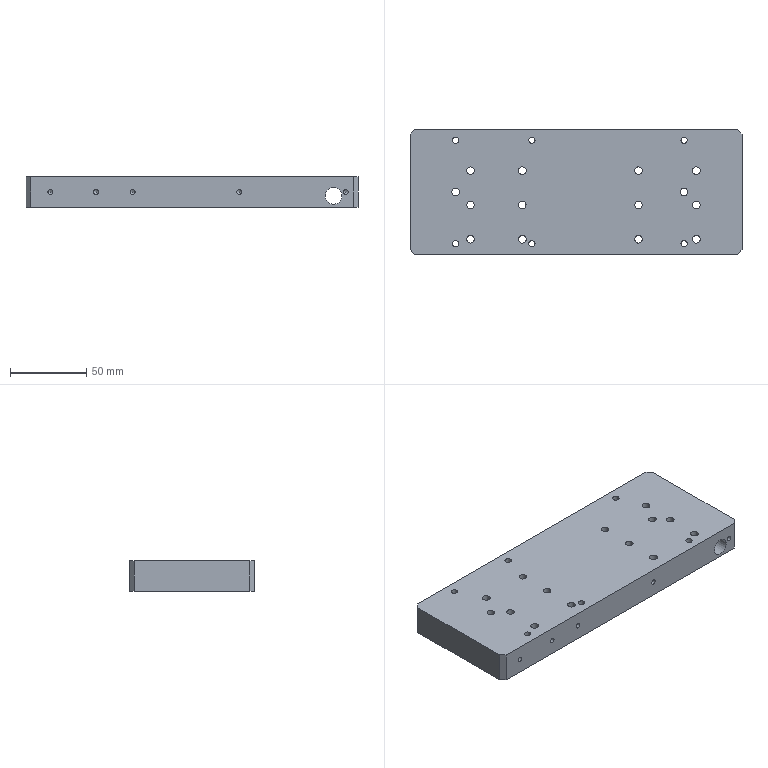Part | 1 solid | 49 faces | box 218 x 82 x 20 mm | volume 338244 mm3 | cylinder 30 | plane 10 | cone 9 | commonest cylinder face diameters 5.1 x8 4.2 x6 5 x6 3.3 x5 6.8 x4 11 x1
STEP:
#1=CARTESIAN_POINT('',(-109.,-38.,10.));
#2=VERTEX_POINT('',#1);
#3=CARTESIAN_POINT('',(-106.,-41.,10.));
#4=VERTEX_POINT('',#3);
#5=CARTESIAN_POINT('',(-106.,-41.,10.));
#6=DIRECTION('',(0.7071,-0.7071,0.));
#7=VECTOR('',#6,1000.);
#8=LINE('',#5,#7);
#9=EDGE_CURVE('',#2,#4,#8,.T.);
#10=ORIENTED_EDGE('',*,*,#9,.F.);
#11=CARTESIAN_POINT('',(-109.,-38.,-10.));
#12=VERTEX_POINT('',#11);
#13=CARTESIAN_POINT('',(-109.,-38.,10.));
#14=DIRECTION('',(0.,0.,1.));
#15=VECTOR('',#14,1000.);
#16=LINE('',#13,#15);
#17=EDGE_CURVE('',#12,#2,#16,.T.);
#18=ORIENTED_EDGE('',*,*,#17,.F.);
#19=CARTESIAN_POINT('',(-106.,-41.,-10.));
#20=VERTEX_POINT('',#19);
#21=CARTESIAN_POINT('',(-73.5,-73.5,-10.));
#22=DIRECTION('',(-0.7071,0.7071,0.));
#23=VECTOR('',#22,1000.);
#24=LINE('',#21,#23);
#25=EDGE_CURVE('',#20,#12,#24,.T.);
#26=ORIENTED_EDGE('',*,*,#25,.F.);
#27=CARTESIAN_POINT('',(-106.,-41.,-10.));
#28=DIRECTION('',(0.,0.,-1.));
#29=VECTOR('',#28,1000.);
#30=LINE('',#27,#29);
#31=EDGE_CURVE('',#4,#20,#30,.T.);
#32=ORIENTED_EDGE('',*,*,#31,.F.);
#33=EDGE_LOOP('',(#10,#18,#26,#32));
#34=FACE_BOUND('',#33,.T.);
#35=CARTESIAN_POINT('',(-106.,-41.,10.));
#36=DIRECTION('',(-0.7071,-0.7071,0.));
#37=DIRECTION('',(0.,0.,1.));
#38=AXIS2_PLACEMENT_3D('',#35,#36,#37);
#39=PLANE('',#38);
#40=ADVANCED_FACE('',(#34),#39,.T.);
#41=CARTESIAN_POINT('',(106.,-41.,10.));
#42=VERTEX_POINT('',#41);
#43=CARTESIAN_POINT('',(109.,-38.,10.));
#44=VERTEX_POINT('',#43);
#45=CARTESIAN_POINT('',(109.,-38.,10.));
#46=DIRECTION('',(0.7071,0.7071,0.));
#47=VECTOR('',#46,1000.);
#48=LINE('',#45,#47);
#49=EDGE_CURVE('',#42,#44,#48,.T.);
#50=ORIENTED_EDGE('',*,*,#49,.F.);
#51=CARTESIAN_POINT('',(106.,-41.,-10.));
#52=VERTEX_POINT('',#51);
#53=CARTESIAN_POINT('',(106.,-41.,10.));
#54=DIRECTION('',(0.,0.,1.));
#55=VECTOR('',#54,1000.);
#56=LINE('',#53,#55);
#57=EDGE_CURVE('',#52,#42,#56,.T.);
#58=ORIENTED_EDGE('',*,*,#57,.F.);
#59=CARTESIAN_POINT('',(109.,-38.,-10.));
#60=VERTEX_POINT('',#59);
#61=CARTESIAN_POINT('',(73.5,-73.5,-10.));
#62=DIRECTION('',(-0.7071,-0.7071,0.));
#63=VECTOR('',#62,1000.);
#64=LINE('',#61,#63);
#65=EDGE_CURVE('',#60,#52,#64,.T.);
#66=ORIENTED_EDGE('',*,*,#65,.F.);
#67=CARTESIAN_POINT('',(109.,-38.,10.));
#68=DIRECTION('',(0.,0.,-1.));
#69=VECTOR('',#68,1000.);
#70=LINE('',#67,#69);
#71=EDGE_CURVE('',#44,#60,#70,.T.);
#72=ORIENTED_EDGE('',*,*,#71,.F.);
#73=EDGE_LOOP('',(#50,#58,#66,#72));
#74=FACE_BOUND('',#73,.T.);
#75=CARTESIAN_POINT('',(109.,-38.,10.));
#76=DIRECTION('',(-0.7071,0.7071,0.));
#77=DIRECTION('',(0.,0.,-1.));
#78=AXIS2_PLACEMENT_3D('',#75,#76,#77);
#79=PLANE('',#78);
#80=ADVANCED_FACE('',(#74),#79,.F.);
#81=CARTESIAN_POINT('',(-106.,41.,10.));
#82=VERTEX_POINT('',#81);
#83=CARTESIAN_POINT('',(-109.,38.,10.));
#84=VERTEX_POINT('',#83);
#85=CARTESIAN_POINT('',(-109.,38.,10.));
#86=DIRECTION('',(-0.7071,-0.7071,0.));
#87=VECTOR('',#86,1000.);
#88=LINE('',#85,#87);
#89=EDGE_CURVE('',#82,#84,#88,.T.);
#90=ORIENTED_EDGE('',*,*,#89,.F.);
#91=CARTESIAN_POINT('',(-106.,41.,-10.));
#92=VERTEX_POINT('',#91);
#93=CARTESIAN_POINT('',(-106.,41.,10.));
#94=DIRECTION('',(0.,0.,1.));
#95=VECTOR('',#94,1000.);
#96=LINE('',#93,#95);
#97=EDGE_CURVE('',#92,#82,#96,.T.);
#98=ORIENTED_EDGE('',*,*,#97,.F.);
#99=CARTESIAN_POINT('',(-109.,38.,-10.));
#100=VERTEX_POINT('',#99);
#101=CARTESIAN_POINT('',(-73.5,73.5,-10.));
#102=DIRECTION('',(0.7071,0.7071,0.));
#103=VECTOR('',#102,1000.);
#104=LINE('',#101,#103);
#105=EDGE_CURVE('',#100,#92,#104,.T.);
#106=ORIENTED_EDGE('',*,*,#105,.F.);
#107=CARTESIAN_POINT('',(-109.,38.,10.));
#108=DIRECTION('',(0.,0.,-1.));
#109=VECTOR('',#108,1000.);
#110=LINE('',#107,#109);
#111=EDGE_CURVE('',#84,#100,#110,.T.);
#112=ORIENTED_EDGE('',*,*,#111,.F.);
#113=EDGE_LOOP('',(#90,#98,#106,#112));
#114=FACE_BOUND('',#113,.T.);
#115=CARTESIAN_POINT('',(-109.,38.,10.));
#116=DIRECTION('',(0.7071,-0.7071,0.));
#117=DIRECTION('',(0.,0.,-1.));
#118=AXIS2_PLACEMENT_3D('',#115,#116,#117);
#119=PLANE('',#118);
#120=ADVANCED_FACE('',(#114),#119,.F.);
#121=CARTESIAN_POINT('',(109.,38.,10.));
#122=VERTEX_POINT('',#121);
#123=CARTESIAN_POINT('',(106.,41.,10.));
#124=VERTEX_POINT('',#123);
#125=CARTESIAN_POINT('',(106.,41.,10.));
#126=DIRECTION('',(-0.7071,0.7071,0.));
#127=VECTOR('',#126,1000.);
#128=LINE('',#125,#127);
#129=EDGE_CURVE('',#122,#124,#128,.T.);
#130=ORIENTED_EDGE('',*,*,#129,.F.);
#131=CARTESIAN_POINT('',(109.,38.,-10.));
#132=VERTEX_POINT('',#131);
#133=CARTESIAN_POINT('',(109.,38.,10.));
#134=DIRECTION('',(0.,0.,1.));
#135=VECTOR('',#134,1000.);
#136=LINE('',#133,#135);
#137=EDGE_CURVE('',#132,#122,#136,.T.);
#138=ORIENTED_EDGE('',*,*,#137,.F.);
#139=CARTESIAN_POINT('',(106.,41.,-10.));
#140=VERTEX_POINT('',#139);
#141=CARTESIAN_POINT('',(73.5,73.5,-10.));
#142=DIRECTION('',(0.7071,-0.7071,0.));
#143=VECTOR('',#142,1000.);
#144=LINE('',#141,#143);
#145=EDGE_CURVE('',#140,#132,#144,.T.);
#146=ORIENTED_EDGE('',*,*,#145,.F.);
#147=CARTESIAN_POINT('',(106.,41.,-10.));
#148=DIRECTION('',(0.,0.,-1.));
#149=VECTOR('',#148,1000.);
#150=LINE('',#147,#149);
#151=EDGE_CURVE('',#124,#140,#150,.T.);
#152=ORIENTED_EDGE('',*,*,#151,.F.);
#153=EDGE_LOOP('',(#130,#138,#146,#152));
#154=FACE_BOUND('',#153,.T.);
#155=CARTESIAN_POINT('',(106.,41.,10.));
#156=DIRECTION('',(0.7071,0.7071,0.));
#157=DIRECTION('',(0.,0.,1.));
#158=AXIS2_PLACEMENT_3D('',#155,#156,#157);
#159=PLANE('',#158);
#160=ADVANCED_FACE('',(#154),#159,.T.);
#161=CARTESIAN_POINT('',(-109.,41.,-10.));
#162=DIRECTION('',(1.,0.,0.));
#163=VECTOR('',#162,1000.);
#164=LINE('',#161,#163);
#165=EDGE_CURVE('',#92,#140,#164,.T.);
#166=ORIENTED_EDGE('',*,*,#165,.T.);
#167=ORIENTED_EDGE('',*,*,#145,.T.);
#168=CARTESIAN_POINT('',(109.,-41.,-10.));
#169=DIRECTION('',(0.,1.,0.));
#170=VECTOR('',#169,1000.);
#171=LINE('',#168,#170);
#172=EDGE_CURVE('',#60,#132,#171,.T.);
#173=ORIENTED_EDGE('',*,*,#172,.F.);
#174=ORIENTED_EDGE('',*,*,#65,.T.);
#175=CARTESIAN_POINT('',(-109.,-41.,-10.));
#176=DIRECTION('',(1.,0.,0.));
#177=VECTOR('',#176,1000.);
#178=LINE('',#175,#177);
#179=EDGE_CURVE('',#20,#52,#178,.T.);
#180=ORIENTED_EDGE('',*,*,#179,.F.);
#181=ORIENTED_EDGE('',*,*,#25,.T.);
#182=CARTESIAN_POINT('',(-109.,-41.,-10.));
#183=DIRECTION('',(0.,1.,0.));
#184=VECTOR('',#183,1000.);
#185=LINE('',#182,#184);
#186=EDGE_CURVE('',#12,#100,#185,.T.);
#187=ORIENTED_EDGE('',*,*,#186,.T.);
#188=ORIENTED_EDGE('',*,*,#105,.T.);
#189=EDGE_LOOP('',(#166,#167,#173,#174,#180,#181,#187,#188));
#190=FACE_BOUND('',#189,.T.);
#191=CARTESIAN_POINT('',(38.45,14.,-10.));
#192=VERTEX_POINT('',#191);
#193=CARTESIAN_POINT('',(41.,14.,-10.));
#194=DIRECTION('',(0.,0.,-1.));
#195=DIRECTION('',(-1.,0.,0.));
#196=AXIS2_PLACEMENT_3D('',#193,#194,#195);
#197=CIRCLE('',#196,2.55);
#198=EDGE_CURVE('',#192,#192,#197,.T.);
#199=ORIENTED_EDGE('',*,*,#198,.F.);
#200=EDGE_LOOP('',(#199));
#201=FACE_BOUND('',#200,.T.);
#202=CARTESIAN_POINT('',(76.45,14.,-10.));
#203=VERTEX_POINT('',#202);
#204=CARTESIAN_POINT('',(79.,14.,-10.));
#205=DIRECTION('',(0.,0.,-1.));
#206=DIRECTION('',(-1.,0.,0.));
#207=AXIS2_PLACEMENT_3D('',#204,#205,#206);
#208=CIRCLE('',#207,2.55);
#209=EDGE_CURVE('',#203,#203,#208,.T.);
#210=ORIENTED_EDGE('',*,*,#209,.F.);
#211=EDGE_LOOP('',(#210));
#212=FACE_BOUND('',#211,.T.);
#213=CARTESIAN_POINT('',(76.45,-31.,-10.));
#214=VERTEX_POINT('',#213);
#215=CARTESIAN_POINT('',(79.,-31.,-10.));
#216=DIRECTION('',(0.,0.,-1.));
#217=DIRECTION('',(-1.,0.,0.));
#218=AXIS2_PLACEMENT_3D('',#215,#216,#217);
#219=CIRCLE('',#218,2.55);
#220=EDGE_CURVE('',#214,#214,#219,.T.);
#221=ORIENTED_EDGE('',*,*,#220,.F.);
#222=EDGE_LOOP('',(#221));
#223=FACE_BOUND('',#222,.T.);
#224=CARTESIAN_POINT('',(38.45,-31.,-10.));
#225=VERTEX_POINT('',#224);
#226=CARTESIAN_POINT('',(41.,-31.,-10.));
#227=DIRECTION('',(0.,0.,-1.));
#228=DIRECTION('',(-1.,0.,0.));
#229=AXIS2_PLACEMENT_3D('',#226,#227,#228);
#230=CIRCLE('',#229,2.55);
#231=EDGE_CURVE('',#225,#225,#230,.T.);
#232=ORIENTED_EDGE('',*,*,#231,.F.);
#233=EDGE_LOOP('',(#232));
#234=FACE_BOUND('',#233,.T.);
#235=CARTESIAN_POINT('',(-31.1,-34.,-10.));
#236=VERTEX_POINT('',#235);
#237=CARTESIAN_POINT('',(-29.,-34.,-10.));
#238=DIRECTION('',(0.,0.,-1.));
#239=DIRECTION('',(-1.,0.,0.));
#240=AXIS2_PLACEMENT_3D('',#237,#238,#239);
#241=CIRCLE('',#240,2.1);
#242=EDGE_CURVE('',#236,#236,#241,.T.);
#243=ORIENTED_EDGE('',*,*,#242,.F.);
#244=EDGE_LOOP('',(#243));
#245=FACE_BOUND('',#244,.T.);
#246=CARTESIAN_POINT('',(-31.1,34.,-10.));
#247=VERTEX_POINT('',#246);
#248=CARTESIAN_POINT('',(-29.,34.,-10.));
#249=DIRECTION('',(0.,0.,-1.));
#250=DIRECTION('',(-1.,0.,0.));
#251=AXIS2_PLACEMENT_3D('',#248,#249,#250);
#252=CIRCLE('',#251,2.1);
#253=EDGE_CURVE('',#247,#247,#252,.T.);
#254=ORIENTED_EDGE('',*,*,#253,.F.);
#255=EDGE_LOOP('',(#254));
#256=FACE_BOUND('',#255,.T.);
#257=CARTESIAN_POINT('',(68.9,34.,-10.));
#258=VERTEX_POINT('',#257);
#259=CARTESIAN_POINT('',(71.,34.,-10.));
#260=DIRECTION('',(0.,0.,-1.));
#261=DIRECTION('',(-1.,0.,0.));
#262=AXIS2_PLACEMENT_3D('',#259,#260,#261);
#263=CIRCLE('',#262,2.1);
#264=EDGE_CURVE('',#258,#258,#263,.T.);
#265=ORIENTED_EDGE('',*,*,#264,.F.);
#266=EDGE_LOOP('',(#265));
#267=FACE_BOUND('',#266,.T.);
#268=CARTESIAN_POINT('',(68.9,-34.,-10.));
#269=VERTEX_POINT('',#268);
#270=CARTESIAN_POINT('',(71.,-34.,-10.));
#271=DIRECTION('',(0.,0.,-1.));
#272=DIRECTION('',(-1.,0.,0.));
#273=AXIS2_PLACEMENT_3D('',#270,#271,#272);
#274=CIRCLE('',#273,2.1);
#275=EDGE_CURVE('',#269,#269,#274,.T.);
#276=ORIENTED_EDGE('',*,*,#275,.F.);
#277=EDGE_LOOP('',(#276));
#278=FACE_BOUND('',#277,.T.);
#279=CARTESIAN_POINT('',(-81.1,34.,-10.));
#280=VERTEX_POINT('',#279);
#281=CARTESIAN_POINT('',(-79.,34.,-10.));
#282=DIRECTION('',(0.,0.,-1.));
#283=DIRECTION('',(-1.,0.,0.));
#284=AXIS2_PLACEMENT_3D('',#281,#282,#283);
#285=CIRCLE('',#284,2.1);
#286=EDGE_CURVE('',#280,#280,#285,.T.);
#287=ORIENTED_EDGE('',*,*,#286,.F.);
#288=EDGE_LOOP('',(#287));
#289=FACE_BOUND('',#288,.T.);
#290=CARTESIAN_POINT('',(-81.1,-34.,-10.));
#291=VERTEX_POINT('',#290);
#292=CARTESIAN_POINT('',(-79.,-34.,-10.));
#293=DIRECTION('',(0.,0.,-1.));
#294=DIRECTION('',(-1.,0.,0.));
#295=AXIS2_PLACEMENT_3D('',#292,#293,#294);
#296=CIRCLE('',#295,2.1);
#297=EDGE_CURVE('',#291,#291,#296,.T.);
#298=ORIENTED_EDGE('',*,*,#297,.F.);
#299=EDGE_LOOP('',(#298));
#300=FACE_BOUND('',#299,.T.);
#301=CARTESIAN_POINT('',(-81.5,0.,-10.));
#302=VERTEX_POINT('',#301);
#303=CARTESIAN_POINT('',(-79.,0.,-10.));
#304=DIRECTION('',(0.,0.,-1.));
#305=DIRECTION('',(-1.,0.,0.));
#306=AXIS2_PLACEMENT_3D('',#303,#304,#305);
#307=CIRCLE('',#306,2.5);
#308=EDGE_CURVE('',#302,#302,#307,.T.);
#309=ORIENTED_EDGE('',*,*,#308,.F.);
#310=EDGE_LOOP('',(#309));
#311=FACE_BOUND('',#310,.T.);
#312=CARTESIAN_POINT('',(68.5,0.,-10.));
#313=VERTEX_POINT('',#312);
#314=CARTESIAN_POINT('',(71.,0.,-10.));
#315=DIRECTION('',(0.,0.,-1.));
#316=DIRECTION('',(-1.,0.,0.));
#317=AXIS2_PLACEMENT_3D('',#314,#315,#316);
#318=CIRCLE('',#317,2.5);
#319=EDGE_CURVE('',#313,#313,#318,.T.);
#320=ORIENTED_EDGE('',*,*,#319,.F.);
#321=EDGE_LOOP('',(#320));
#322=FACE_BOUND('',#321,.T.);
#323=CARTESIAN_POINT('',(38.5,-8.5,-10.));
#324=VERTEX_POINT('',#323);
#325=CARTESIAN_POINT('',(41.,-8.5,-10.));
#326=DIRECTION('',(0.,0.,-1.));
#327=DIRECTION('',(-1.,0.,0.));
#328=AXIS2_PLACEMENT_3D('',#325,#326,#327);
#329=CIRCLE('',#328,2.5);
#330=EDGE_CURVE('',#324,#324,#329,.T.);
#331=ORIENTED_EDGE('',*,*,#330,.F.);
#332=EDGE_LOOP('',(#331));
#333=FACE_BOUND('',#332,.T.);
#334=CARTESIAN_POINT('',(76.5,-8.5,-10.));
#335=VERTEX_POINT('',#334);
#336=CARTESIAN_POINT('',(79.,-8.5,-10.));
#337=DIRECTION('',(0.,0.,-1.));
#338=DIRECTION('',(-1.,0.,0.));
#339=AXIS2_PLACEMENT_3D('',#336,#337,#338);
#340=CIRCLE('',#339,2.5);
#341=EDGE_CURVE('',#335,#335,#340,.T.);
#342=ORIENTED_EDGE('',*,*,#341,.F.);
#343=EDGE_LOOP('',(#342));
#344=FACE_BOUND('',#343,.T.);
#345=CARTESIAN_POINT('',(-37.825,14.,-10.));
#346=VERTEX_POINT('',#345);
#347=CARTESIAN_POINT('',(-35.275,14.,-10.));
#348=DIRECTION('',(0.,0.,-1.));
#349=DIRECTION('',(-1.,0.,0.));
#350=AXIS2_PLACEMENT_3D('',#347,#348,#349);
#351=CIRCLE('',#350,2.55);
#352=EDGE_CURVE('',#346,#346,#351,.T.);
#353=ORIENTED_EDGE('',*,*,#352,.F.);
#354=EDGE_LOOP('',(#353));
#355=FACE_BOUND('',#354,.T.);
#356=CARTESIAN_POINT('',(-71.825,14.,-10.));
#357=VERTEX_POINT('',#356);
#358=CARTESIAN_POINT('',(-69.275,14.,-10.));
#359=DIRECTION('',(0.,0.,-1.));
#360=DIRECTION('',(-1.,0.,0.));
#361=AXIS2_PLACEMENT_3D('',#358,#359,#360);
#362=CIRCLE('',#361,2.55);
#363=EDGE_CURVE('',#357,#357,#362,.T.);
#364=ORIENTED_EDGE('',*,*,#363,.F.);
#365=EDGE_LOOP('',(#364));
#366=FACE_BOUND('',#365,.T.);
#367=CARTESIAN_POINT('',(-37.825,-31.,-10.));
#368=VERTEX_POINT('',#367);
#369=CARTESIAN_POINT('',(-35.275,-31.,-10.));
#370=DIRECTION('',(0.,0.,-1.));
#371=DIRECTION('',(-1.,0.,0.));
#372=AXIS2_PLACEMENT_3D('',#369,#370,#371);
#373=CIRCLE('',#372,2.55);
#374=EDGE_CURVE('',#368,#368,#373,.T.);
#375=ORIENTED_EDGE('',*,*,#374,.F.);
#376=EDGE_LOOP('',(#375));
#377=FACE_BOUND('',#376,.T.);
#378=CARTESIAN_POINT('',(-71.825,-31.,-10.));
#379=VERTEX_POINT('',#378);
#380=CARTESIAN_POINT('',(-69.275,-31.,-10.));
#381=DIRECTION('',(0.,0.,-1.));
#382=DIRECTION('',(-1.,0.,0.));
#383=AXIS2_PLACEMENT_3D('',#380,#381,#382);
#384=CIRCLE('',#383,2.55);
#385=EDGE_CURVE('',#379,#379,#384,.T.);
#386=ORIENTED_EDGE('',*,*,#385,.F.);
#387=EDGE_LOOP('',(#386));
#388=FACE_BOUND('',#387,.T.);
#389=CARTESIAN_POINT('',(-37.775,-8.5,-10.));
#390=VERTEX_POINT('',#389);
#391=CARTESIAN_POINT('',(-35.275,-8.5,-10.));
#392=DIRECTION('',(0.,0.,-1.));
#393=DIRECTION('',(-1.,0.,0.));
#394=AXIS2_PLACEMENT_3D('',#391,#392,#393);
#395=CIRCLE('',#394,2.5);
#396=EDGE_CURVE('',#390,#390,#395,.T.);
#397=ORIENTED_EDGE('',*,*,#396,.F.);
#398=EDGE_LOOP('',(#397));
#399=FACE_BOUND('',#398,.T.);
#400=CARTESIAN_POINT('',(-71.775,-8.5,-10.));
#401=VERTEX_POINT('',#400);
#402=CARTESIAN_POINT('',(-69.275,-8.5,-10.));
#403=DIRECTION('',(0.,0.,-1.));
#404=DIRECTION('',(-1.,0.,0.));
#405=AXIS2_PLACEMENT_3D('',#402,#403,#404);
#406=CIRCLE('',#405,2.5);
#407=EDGE_CURVE('',#401,#401,#406,.T.);
#408=ORIENTED_EDGE('',*,*,#407,.F.);
#409=EDGE_LOOP('',(#408));
#410=FACE_BOUND('',#409,.T.);
#411=CARTESIAN_POINT('',(0.,0.,-10.));
#412=DIRECTION('',(0.,0.,-1.));
#413=DIRECTION('',(-1.,0.,0.));
#414=AXIS2_PLACEMENT_3D('',#411,#412,#413);
#415=PLANE('',#414);
#416=ADVANCED_FACE('',(#190,#201,#212,#223,#234,#245,#256,#267,#278,#289,#300,#311,#322,#333,#344,#355,#366,#377,#388,#399,#410),#415,.T.);
#417=CARTESIAN_POINT('',(109.,-41.,10.));
#418=DIRECTION('',(0.,1.,0.));
#419=VECTOR('',#418,1000.);
#420=LINE('',#417,#419);
#421=EDGE_CURVE('',#44,#122,#420,.T.);
#422=ORIENTED_EDGE('',*,*,#421,.T.);
#423=ORIENTED_EDGE('',*,*,#129,.T.);
#424=CARTESIAN_POINT('',(-109.,41.,10.));
#425=DIRECTION('',(1.,0.,0.));
#426=VECTOR('',#425,1000.);
#427=LINE('',#424,#426);
#428=EDGE_CURVE('',#82,#124,#427,.T.);
#429=ORIENTED_EDGE('',*,*,#428,.F.);
#430=ORIENTED_EDGE('',*,*,#89,.T.);
#431=CARTESIAN_POINT('',(-109.,-41.,10.));
#432=DIRECTION('',(0.,1.,0.));
#433=VECTOR('',#432,1000.);
#434=LINE('',#431,#433);
#435=EDGE_CURVE('',#2,#84,#434,.T.);
#436=ORIENTED_EDGE('',*,*,#435,.F.);
#437=ORIENTED_EDGE('',*,*,#9,.T.);
#438=CARTESIAN_POINT('',(-109.,-41.,10.));
#439=DIRECTION('',(1.,0.,0.));
#440=VECTOR('',#439,1000.);
#441=LINE('',#438,#440);
#442=EDGE_CURVE('',#4,#42,#441,.T.);
#443=ORIENTED_EDGE('',*,*,#442,.T.);
#444=ORIENTED_EDGE('',*,*,#49,.T.);
#445=EDGE_LOOP('',(#422,#423,#429,#430,#436,#437,#443,#444));
#446=FACE_BOUND('',#445,.T.);
#447=CARTESIAN_POINT('',(38.45,14.,10.));
#448=VERTEX_POINT('',#447);
#449=CARTESIAN_POINT('',(41.,14.,10.));
#450=DIRECTION('',(0.,0.,-1.));
#451=DIRECTION('',(-1.,0.,0.));
#452=AXIS2_PLACEMENT_3D('',#449,#450,#451);
#453=CIRCLE('',#452,2.55);
#454=EDGE_CURVE('',#448,#448,#453,.T.);
#455=ORIENTED_EDGE('',*,*,#454,.T.);
#456=EDGE_LOOP('',(#455));
#457=FACE_BOUND('',#456,.T.);
#458=CARTESIAN_POINT('',(76.45,14.,10.));
#459=VERTEX_POINT('',#458);
#460=CARTESIAN_POINT('',(79.,14.,10.));
#461=DIRECTION('',(0.,0.,-1.));
#462=DIRECTION('',(-1.,0.,0.));
#463=AXIS2_PLACEMENT_3D('',#460,#461,#462);
#464=CIRCLE('',#463,2.55);
#465=EDGE_CURVE('',#459,#459,#464,.T.);
#466=ORIENTED_EDGE('',*,*,#465,.T.);
#467=EDGE_LOOP('',(#466));
#468=FACE_BOUND('',#467,.T.);
#469=CARTESIAN_POINT('',(76.45,-31.,10.));
#470=VERTEX_POINT('',#469);
#471=CARTESIAN_POINT('',(79.,-31.,10.));
#472=DIRECTION('',(0.,0.,-1.));
#473=DIRECTION('',(-1.,0.,0.));
#474=AXIS2_PLACEMENT_3D('',#471,#472,#473);
#475=CIRCLE('',#474,2.55);
#476=EDGE_CURVE('',#470,#470,#475,.T.);
#477=ORIENTED_EDGE('',*,*,#476,.T.);
#478=EDGE_LOOP('',(#477));
#479=FACE_BOUND('',#478,.T.);
#480=CARTESIAN_POINT('',(38.45,-31.,10.));
#481=VERTEX_POINT('',#480);
#482=CARTESIAN_POINT('',(41.,-31.,10.));
#483=DIRECTION('',(0.,0.,-1.));
#484=DIRECTION('',(-1.,0.,0.));
#485=AXIS2_PLACEMENT_3D('',#482,#483,#484);
#486=CIRCLE('',#485,2.55);
#487=EDGE_CURVE('',#481,#481,#486,.T.);
#488=ORIENTED_EDGE('',*,*,#487,.T.);
#489=EDGE_LOOP('',(#488));
#490=FACE_BOUND('',#489,.T.);
#491=CARTESIAN_POINT('',(-31.1,-34.,10.));
#492=VERTEX_POINT('',#491);
#493=CARTESIAN_POINT('',(-29.,-34.,10.));
#494=DIRECTION('',(0.,0.,-1.));
#495=DIRECTION('',(-1.,0.,0.));
#496=AXIS2_PLACEMENT_3D('',#493,#494,#495);
#497=CIRCLE('',#496,2.1);
#498=EDGE_CURVE('',#492,#492,#497,.T.);
#499=ORIENTED_EDGE('',*,*,#498,.T.);
#500=EDGE_LOOP('',(#499));
#501=FACE_BOUND('',#500,.T.);
#502=CARTESIAN_POINT('',(-31.1,34.,10.));
#503=VERTEX_POINT('',#502);
#504=CARTESIAN_POINT('',(-29.,34.,10.));
#505=DIRECTION('',(0.,0.,-1.));
#506=DIRECTION('',(-1.,0.,0.));
#507=AXIS2_PLACEMENT_3D('',#504,#505,#506);
#508=CIRCLE('',#507,2.1);
#509=EDGE_CURVE('',#503,#503,#508,.T.);
#510=ORIENTED_EDGE('',*,*,#509,.T.);
#511=EDGE_LOOP('',(#510));
#512=FACE_BOUND('',#511,.T.);
#513=CARTESIAN_POINT('',(68.9,34.,10.));
#514=VERTEX_POINT('',#513);
#515=CARTESIAN_POINT('',(71.,34.,10.));
#516=DIRECTION('',(0.,0.,-1.));
#517=DIRECTION('',(-1.,0.,0.));
#518=AXIS2_PLACEMENT_3D('',#515,#516,#517);
#519=CIRCLE('',#518,2.1);
#520=EDGE_CURVE('',#514,#514,#519,.T.);
#521=ORIENTED_EDGE('',*,*,#520,.T.);
#522=EDGE_LOOP('',(#521));
#523=FACE_BOUND('',#522,.T.);
#524=CARTESIAN_POINT('',(68.9,-34.,10.));
#525=VERTEX_POINT('',#524);
#526=CARTESIAN_POINT('',(71.,-34.,10.));
#527=DIRECTION('',(0.,0.,-1.));
#528=DIRECTION('',(-1.,0.,0.));
#529=AXIS2_PLACEMENT_3D('',#526,#527,#528);
#530=CIRCLE('',#529,2.1);
#531=EDGE_CURVE('',#525,#525,#530,.T.);
#532=ORIENTED_EDGE('',*,*,#531,.T.);
#533=EDGE_LOOP('',(#532));
#534=FACE_BOUND('',#533,.T.);
#535=CARTESIAN_POINT('',(-81.1,34.,10.));
#536=VERTEX_POINT('',#535);
#537=CARTESIAN_POINT('',(-79.,34.,10.));
#538=DIRECTION('',(0.,0.,-1.));
#539=DIRECTION('',(-1.,0.,0.));
#540=AXIS2_PLACEMENT_3D('',#537,#538,#539);
#541=CIRCLE('',#540,2.1);
#542=EDGE_CURVE('',#536,#536,#541,.T.);
#543=ORIENTED_EDGE('',*,*,#542,.T.);
#544=EDGE_LOOP('',(#543));
#545=FACE_BOUND('',#544,.T.);
#546=CARTESIAN_POINT('',(-81.1,-34.,10.));
#547=VERTEX_POINT('',#546);
#548=CARTESIAN_POINT('',(-79.,-34.,10.));
#549=DIRECTION('',(0.,0.,-1.));
#550=DIRECTION('',(-1.,0.,0.));
#551=AXIS2_PLACEMENT_3D('',#548,#549,#550);
#552=CIRCLE('',#551,2.1);
#553=EDGE_CURVE('',#547,#547,#552,.T.);
#554=ORIENTED_EDGE('',*,*,#553,.T.);
#555=EDGE_LOOP('',(#554));
#556=FACE_BOUND('',#555,.T.);
#557=CARTESIAN_POINT('',(-81.5,0.,10.));
#558=VERTEX_POINT('',#557);
#559=CARTESIAN_POINT('',(-79.,0.,10.));
#560=DIRECTION('',(0.,0.,-1.));
#561=DIRECTION('',(-1.,0.,0.));
#562=AXIS2_PLACEMENT_3D('',#559,#560,#561);
#563=CIRCLE('',#562,2.5);
#564=EDGE_CURVE('',#558,#558,#563,.T.);
#565=ORIENTED_EDGE('',*,*,#564,.T.);
#566=EDGE_LOOP('',(#565));
#567=FACE_BOUND('',#566,.T.);
#568=CARTESIAN_POINT('',(68.5,0.,10.));
#569=VERTEX_POINT('',#568);
#570=CARTESIAN_POINT('',(71.,0.,10.));
#571=DIRECTION('',(0.,0.,-1.));
#572=DIRECTION('',(-1.,0.,0.));
#573=AXIS2_PLACEMENT_3D('',#570,#571,#572);
#574=CIRCLE('',#573,2.5);
#575=EDGE_CURVE('',#569,#569,#574,.T.);
#576=ORIENTED_EDGE('',*,*,#575,.T.);
#577=EDGE_LOOP('',(#576));
#578=FACE_BOUND('',#577,.T.);
#579=CARTESIAN_POINT('',(38.5,-8.5,10.));
#580=VERTEX_POINT('',#579);
#581=CARTESIAN_POINT('',(41.,-8.5,10.));
#582=DIRECTION('',(0.,0.,-1.));
#583=DIRECTION('',(-1.,0.,0.));
#584=AXIS2_PLACEMENT_3D('',#581,#582,#583);
#585=CIRCLE('',#584,2.5);
#586=EDGE_CURVE('',#580,#580,#585,.T.);
#587=ORIENTED_EDGE('',*,*,#586,.T.);
#588=EDGE_LOOP('',(#587));
#589=FACE_BOUND('',#588,.T.);
#590=CARTESIAN_POINT('',(76.5,-8.5,10.));
#591=VERTEX_POINT('',#590);
#592=CARTESIAN_POINT('',(79.,-8.5,10.));
#593=DIRECTION('',(0.,0.,-1.));
#594=DIRECTION('',(-1.,0.,0.));
#595=AXIS2_PLACEMENT_3D('',#592,#593,#594);
#596=CIRCLE('',#595,2.5);
#597=EDGE_CURVE('',#591,#591,#596,.T.);
#598=ORIENTED_EDGE('',*,*,#597,.T.);
#599=EDGE_LOOP('',(#598));
#600=FACE_BOUND('',#599,.T.);
#601=CARTESIAN_POINT('',(-37.825,14.,10.));
#602=VERTEX_POINT('',#601);
#603=CARTESIAN_POINT('',(-35.275,14.,10.));
#604=DIRECTION('',(0.,0.,-1.));
#605=DIRECTION('',(-1.,0.,0.));
#606=AXIS2_PLACEMENT_3D('',#603,#604,#605);
#607=CIRCLE('',#606,2.55);
#608=EDGE_CURVE('',#602,#602,#607,.T.);
#609=ORIENTED_EDGE('',*,*,#608,.T.);
#610=EDGE_LOOP('',(#609));
#611=FACE_BOUND('',#610,.T.);
#612=CARTESIAN_POINT('',(-71.825,14.,10.));
#613=VERTEX_POINT('',#612);
#614=CARTESIAN_POINT('',(-69.275,14.,10.));
#615=DIRECTION('',(0.,0.,-1.));
#616=DIRECTION('',(-1.,0.,0.));
#617=AXIS2_PLACEMENT_3D('',#614,#615,#616);
#618=CIRCLE('',#617,2.55);
#619=EDGE_CURVE('',#613,#613,#618,.T.);
#620=ORIENTED_EDGE('',*,*,#619,.T.);
#621=EDGE_LOOP('',(#620));
#622=FACE_BOUND('',#621,.T.);
#623=CARTESIAN_POINT('',(-37.825,-31.,10.));
#624=VERTEX_POINT('',#623);
#625=CARTESIAN_POINT('',(-35.275,-31.,10.));
#626=DIRECTION('',(0.,0.,-1.));
#627=DIRECTION('',(-1.,0.,0.));
#628=AXIS2_PLACEMENT_3D('',#625,#626,#627);
#629=CIRCLE('',#628,2.55);
#630=EDGE_CURVE('',#624,#624,#629,.T.);
#631=ORIENTED_EDGE('',*,*,#630,.T.);
#632=EDGE_LOOP('',(#631));
#633=FACE_BOUND('',#632,.T.);
#634=CARTESIAN_POINT('',(-71.825,-31.,10.));
#635=VERTEX_POINT('',#634);
#636=CARTESIAN_POINT('',(-69.275,-31.,10.));
#637=DIRECTION('',(0.,0.,-1.));
#638=DIRECTION('',(-1.,0.,0.));
#639=AXIS2_PLACEMENT_3D('',#636,#637,#638);
#640=CIRCLE('',#639,2.55);
#641=EDGE_CURVE('',#635,#635,#640,.T.);
#642=ORIENTED_EDGE('',*,*,#641,.T.);
#643=EDGE_LOOP('',(#642));
#644=FACE_BOUND('',#643,.T.);
#645=CARTESIAN_POINT('',(-37.775,-8.5,10.));
#646=VERTEX_POINT('',#645);
#647=CARTESIAN_POINT('',(-35.275,-8.5,10.));
#648=DIRECTION('',(0.,0.,-1.));
#649=DIRECTION('',(-1.,0.,0.));
#650=AXIS2_PLACEMENT_3D('',#647,#648,#649);
#651=CIRCLE('',#650,2.5);
#652=EDGE_CURVE('',#646,#646,#651,.T.);
#653=ORIENTED_EDGE('',*,*,#652,.T.);
#654=EDGE_LOOP('',(#653));
#655=FACE_BOUND('',#654,.T.);
#656=CARTESIAN_POINT('',(-71.775,-8.5,10.));
#657=VERTEX_POINT('',#656);
#658=CARTESIAN_POINT('',(-69.275,-8.5,10.));
#659=DIRECTION('',(0.,0.,-1.));
#660=DIRECTION('',(-1.,0.,0.));
#661=AXIS2_PLACEMENT_3D('',#658,#659,#660);
#662=CIRCLE('',#661,2.5);
#663=EDGE_CURVE('',#657,#657,#662,.T.);
#664=ORIENTED_EDGE('',*,*,#663,.T.);
#665=EDGE_LOOP('',(#664));
#666=FACE_BOUND('',#665,.T.);
#667=CARTESIAN_POINT('',(0.,0.,10.));
#668=DIRECTION('',(0.,0.,-1.));
#669=DIRECTION('',(-1.,0.,0.));
#670=AXIS2_PLACEMENT_3D('',#667,#668,#669);
#671=PLANE('',#670);
#672=ADVANCED_FACE('',(#446,#457,#468,#479,#490,#501,#512,#523,#534,#545,#556,#567,#578,#589,#600,#611,#622,#633,#644,#655,#666),#671,.F.);
#673=ORIENTED_EDGE('',*,*,#428,.T.);
#674=ORIENTED_EDGE('',*,*,#151,.T.);
#675=ORIENTED_EDGE('',*,*,#165,.F.);
#676=ORIENTED_EDGE('',*,*,#97,.T.);
#677=EDGE_LOOP('',(#673,#674,#675,#676));
#678=FACE_BOUND('',#677,.T.);
#679=CARTESIAN_POINT('',(-44.,41.,3.4));
#680=VERTEX_POINT('',#679);
#681=CARTESIAN_POINT('',(-44.,41.,0.));
#682=DIRECTION('',(0.,1.,0.));
#683=DIRECTION('',(0.,0.,1.));
#684=AXIS2_PLACEMENT_3D('',#681,#682,#683);
#685=CIRCLE('',#684,3.4);
#686=EDGE_CURVE('',#680,#680,#685,.T.);
#687=ORIENTED_EDGE('',*,*,#686,.F.);
#688=EDGE_LOOP('',(#687));
#689=FACE_BOUND('',#688,.T.);
#690=CARTESIAN_POINT('',(61.,41.,3.4));
#691=VERTEX_POINT('',#690);
#692=CARTESIAN_POINT('',(61.,41.,0.));
#693=DIRECTION('',(0.,1.,0.));
#694=DIRECTION('',(0.,0.,1.));
#695=AXIS2_PLACEMENT_3D('',#692,#693,#694);
#696=CIRCLE('',#695,3.4);
#697=EDGE_CURVE('',#691,#691,#696,.T.);
#698=ORIENTED_EDGE('',*,*,#697,.F.);
#699=EDGE_LOOP('',(#698));
#700=FACE_BOUND('',#699,.T.);
#701=CARTESIAN_POINT('',(11.,41.,3.4));
#702=VERTEX_POINT('',#701);
#703=CARTESIAN_POINT('',(11.,41.,0.));
#704=DIRECTION('',(0.,1.,0.));
#705=DIRECTION('',(0.,0.,1.));
#706=AXIS2_PLACEMENT_3D('',#703,#704,#705);
#707=CIRCLE('',#706,3.4);
#708=EDGE_CURVE('',#702,#702,#707,.T.);
#709=ORIENTED_EDGE('',*,*,#708,.F.);
#710=EDGE_LOOP('',(#709));
#711=FACE_BOUND('',#710,.T.);
#712=CARTESIAN_POINT('',(-99.,41.,3.4));
#713=VERTEX_POINT('',#712);
#714=CARTESIAN_POINT('',(-99.,41.,0.));
#715=DIRECTION('',(0.,1.,0.));
#716=DIRECTION('',(0.,0.,1.));
#717=AXIS2_PLACEMENT_3D('',#714,#715,#716);
#718=CIRCLE('',#717,3.4);
#719=EDGE_CURVE('',#713,#713,#718,.T.);
#720=ORIENTED_EDGE('',*,*,#719,.F.);
#721=EDGE_LOOP('',(#720));
#722=FACE_BOUND('',#721,.T.);
#723=CARTESIAN_POINT('',(93.,41.,-8.));
#724=VERTEX_POINT('',#723);
#725=CARTESIAN_POINT('',(93.,41.,-2.5));
#726=DIRECTION('',(0.,-1.,0.));
#727=DIRECTION('',(0.,0.,-1.));
#728=AXIS2_PLACEMENT_3D('',#725,#726,#727);
#729=CIRCLE('',#728,5.5);
#730=EDGE_CURVE('',#724,#724,#729,.T.);
#731=ORIENTED_EDGE('',*,*,#730,.T.);
#732=EDGE_LOOP('',(#731));
#733=FACE_BOUND('',#732,.T.);
#734=CARTESIAN_POINT('',(-109.,41.,10.));
#735=DIRECTION('',(0.,1.,0.));
#736=DIRECTION('',(0.,0.,1.));
#737=AXIS2_PLACEMENT_3D('',#734,#735,#736);
#738=PLANE('',#737);
#739=ADVANCED_FACE('',(#678,#689,#700,#711,#722,#733),#738,.T.);
#740=ORIENTED_EDGE('',*,*,#172,.T.);
#741=ORIENTED_EDGE('',*,*,#137,.T.);
#742=ORIENTED_EDGE('',*,*,#421,.F.);
#743=ORIENTED_EDGE('',*,*,#71,.T.);
#744=EDGE_LOOP('',(#740,#741,#742,#743));
#745=FACE_BOUND('',#744,.T.);
#746=CARTESIAN_POINT('',(109.,-41.,10.));
#747=DIRECTION('',(-1.,0.,0.));
#748=DIRECTION('',(0.,0.,1.));
#749=AXIS2_PLACEMENT_3D('',#746,#747,#748);
#750=PLANE('',#749);
#751=ADVANCED_FACE('',(#745),#750,.F.);
#752=ORIENTED_EDGE('',*,*,#179,.T.);
#753=ORIENTED_EDGE('',*,*,#57,.T.);
#754=ORIENTED_EDGE('',*,*,#442,.F.);
#755=ORIENTED_EDGE('',*,*,#31,.T.);
#756=EDGE_LOOP('',(#752,#753,#754,#755));
#757=FACE_BOUND('',#756,.T.);
#758=CARTESIAN_POINT('',(101.,-41.,-1.65));
#759=VERTEX_POINT('',#758);
#760=CARTESIAN_POINT('',(101.,-41.,0.));
#761=DIRECTION('',(0.,-1.,0.));
#762=DIRECTION('',(0.,0.,-1.));
#763=AXIS2_PLACEMENT_3D('',#760,#761,#762);
#764=CIRCLE('',#763,1.65);
#765=EDGE_CURVE('',#759,#759,#764,.T.);
#766=ORIENTED_EDGE('',*,*,#765,.F.);
#767=EDGE_LOOP('',(#766));
#768=FACE_BOUND('',#767,.T.);
#769=CARTESIAN_POINT('',(31.,-41.,-1.65));
#770=VERTEX_POINT('',#769);
#771=CARTESIAN_POINT('',(31.,-41.,0.));
#772=DIRECTION('',(0.,-1.,0.));
#773=DIRECTION('',(0.,0.,-1.));
#774=AXIS2_PLACEMENT_3D('',#771,#772,#773);
#775=CIRCLE('',#774,1.65);
#776=EDGE_CURVE('',#770,#770,#775,.T.);
#777=ORIENTED_EDGE('',*,*,#776,.F.);
#778=EDGE_LOOP('',(#777));
#779=FACE_BOUND('',#778,.T.);
#780=CARTESIAN_POINT('',(-39.,-41.,-1.65));
#781=VERTEX_POINT('',#780);
#782=CARTESIAN_POINT('',(-39.,-41.,0.));
#783=DIRECTION('',(0.,-1.,0.));
#784=DIRECTION('',(0.,0.,-1.));
#785=AXIS2_PLACEMENT_3D('',#782,#783,#784);
#786=CIRCLE('',#785,1.65);
#787=EDGE_CURVE('',#781,#781,#786,.T.);
#788=ORIENTED_EDGE('',*,*,#787,.F.);
#789=EDGE_LOOP('',(#788));
#790=FACE_BOUND('',#789,.T.);
#791=CARTESIAN_POINT('',(-63.,-41.,-1.65));
#792=VERTEX_POINT('',#791);
#793=CARTESIAN_POINT('',(-63.,-41.,0.));
#794=DIRECTION('',(0.,-1.,0.));
#795=DIRECTION('',(0.,0.,-1.));
#796=AXIS2_PLACEMENT_3D('',#793,#794,#795);
#797=CIRCLE('',#796,1.65);
#798=EDGE_CURVE('',#792,#792,#797,.T.);
#799=ORIENTED_EDGE('',*,*,#798,.F.);
#800=EDGE_LOOP('',(#799));
#801=FACE_BOUND('',#800,.T.);
#802=CARTESIAN_POINT('',(-93.,-41.,-1.65));
#803=VERTEX_POINT('',#802);
#804=CARTESIAN_POINT('',(-93.,-41.,0.));
#805=DIRECTION('',(0.,-1.,0.));
#806=DIRECTION('',(0.,0.,-1.));
#807=AXIS2_PLACEMENT_3D('',#804,#805,#806);
#808=CIRCLE('',#807,1.65);
#809=EDGE_CURVE('',#803,#803,#808,.T.);
#810=ORIENTED_EDGE('',*,*,#809,.F.);
#811=EDGE_LOOP('',(#810));
#812=FACE_BOUND('',#811,.T.);
#813=CARTESIAN_POINT('',(93.,-41.,-8.));
#814=VERTEX_POINT('',#813);
#815=CARTESIAN_POINT('',(93.,-41.,-2.5));
#816=DIRECTION('',(0.,-1.,0.));
#817=DIRECTION('',(0.,0.,-1.));
#818=AXIS2_PLACEMENT_3D('',#815,#816,#817);
#819=CIRCLE('',#818,5.5);
#820=EDGE_CURVE('',#814,#814,#819,.T.);
#821=ORIENTED_EDGE('',*,*,#820,.F.);
#822=EDGE_LOOP('',(#821));
#823=FACE_BOUND('',#822,.T.);
#824=CARTESIAN_POINT('',(-109.,-41.,10.));
#825=DIRECTION('',(0.,1.,0.));
#826=DIRECTION('',(0.,0.,1.));
#827=AXIS2_PLACEMENT_3D('',#824,#825,#826);
#828=PLANE('',#827);
#829=ADVANCED_FACE('',(#757,#768,#779,#790,#801,#812,#823),#828,.F.);
#830=ORIENTED_EDGE('',*,*,#435,.T.);
#831=ORIENTED_EDGE('',*,*,#111,.T.);
#832=ORIENTED_EDGE('',*,*,#186,.F.);
#833=ORIENTED_EDGE('',*,*,#17,.T.);
#834=EDGE_LOOP('',(#830,#831,#832,#833));
#835=FACE_BOUND('',#834,.T.);
#836=CARTESIAN_POINT('',(-109.,-41.,10.));
#837=DIRECTION('',(-1.,0.,0.));
#838=DIRECTION('',(0.,0.,1.));
#839=AXIS2_PLACEMENT_3D('',#836,#837,#838);
#840=PLANE('',#839);
#841=ADVANCED_FACE('',(#835),#840,.T.);
#842=CARTESIAN_POINT('',(-44.,18.75,3.4));
#843=VERTEX_POINT('',#842);
#844=CARTESIAN_POINT('',(-44.,18.75,0.));
#845=DIRECTION('',(0.,1.,0.));
#846=DIRECTION('',(0.,0.,1.));
#847=AXIS2_PLACEMENT_3D('',#844,#845,#846);
#848=CIRCLE('',#847,3.4);
#849=EDGE_CURVE('',#843,#843,#848,.T.);
#850=ORIENTED_EDGE('',*,*,#849,.T.);
#851=EDGE_LOOP('',(#850));
#852=FACE_BOUND('',#851,.T.);
#853=CARTESIAN_POINT('',(-44.,16.707,0.));
#854=VERTEX_POINT('',#853);
#855=VERTEX_LOOP('',#854);
#856=FACE_BOUND('',#855,.T.);
#857=CARTESIAN_POINT('',(-44.,18.75,0.));
#858=DIRECTION('',(0.,1.,0.));
#859=DIRECTION('',(0.,0.,1.));
#860=AXIS2_PLACEMENT_3D('',#857,#858,#859);
#861=CONICAL_SURFACE('',#860,3.4,1.03);
#862=ADVANCED_FACE('',(#852,#856),#861,.F.);
#863=ORIENTED_EDGE('',*,*,#849,.F.);
#864=EDGE_LOOP('',(#863));
#865=FACE_BOUND('',#864,.T.);
#866=ORIENTED_EDGE('',*,*,#686,.T.);
#867=EDGE_LOOP('',(#866));
#868=FACE_BOUND('',#867,.T.);
#869=CARTESIAN_POINT('',(-44.,41.,0.));
#870=DIRECTION('',(0.,1.,0.));
#871=DIRECTION('',(0.,0.,1.));
#872=AXIS2_PLACEMENT_3D('',#869,#870,#871);
#873=CYLINDRICAL_SURFACE('',#872,3.4);
#874=ADVANCED_FACE('',(#865,#868),#873,.F.);
#875=CARTESIAN_POINT('',(61.,18.75,3.4));
#876=VERTEX_POINT('',#875);
#877=CARTESIAN_POINT('',(61.,18.75,0.));
#878=DIRECTION('',(0.,1.,0.));
#879=DIRECTION('',(0.,0.,1.));
#880=AXIS2_PLACEMENT_3D('',#877,#878,#879);
#881=CIRCLE('',#880,3.4);
#882=EDGE_CURVE('',#876,#876,#881,.T.);
#883=ORIENTED_EDGE('',*,*,#882,.T.);
#884=EDGE_LOOP('',(#883));
#885=FACE_BOUND('',#884,.T.);
#886=CARTESIAN_POINT('',(61.,16.707,0.));
#887=VERTEX_POINT('',#886);
#888=VERTEX_LOOP('',#887);
#889=FACE_BOUND('',#888,.T.);
#890=CARTESIAN_POINT('',(61.,18.75,0.));
#891=DIRECTION('',(0.,1.,0.));
#892=DIRECTION('',(0.,0.,1.));
#893=AXIS2_PLACEMENT_3D('',#890,#891,#892);
#894=CONICAL_SURFACE('',#893,3.4,1.03);
#895=ADVANCED_FACE('',(#885,#889),#894,.F.);
#896=ORIENTED_EDGE('',*,*,#882,.F.);
#897=EDGE_LOOP('',(#896));
#898=FACE_BOUND('',#897,.T.);
#899=ORIENTED_EDGE('',*,*,#697,.T.);
#900=EDGE_LOOP('',(#899));
#901=FACE_BOUND('',#900,.T.);
#902=CARTESIAN_POINT('',(61.,41.,0.));
#903=DIRECTION('',(0.,1.,0.));
#904=DIRECTION('',(0.,0.,1.));
#905=AXIS2_PLACEMENT_3D('',#902,#903,#904);
#906=CYLINDRICAL_SURFACE('',#905,3.4);
#907=ADVANCED_FACE('',(#898,#901),#906,.F.);
#908=CARTESIAN_POINT('',(11.,18.75,3.4));
#909=VERTEX_POINT('',#908);
#910=CARTESIAN_POINT('',(11.,18.75,0.));
#911=DIRECTION('',(0.,1.,0.));
#912=DIRECTION('',(0.,0.,1.));
#913=AXIS2_PLACEMENT_3D('',#910,#911,#912);
#914=CIRCLE('',#913,3.4);
#915=EDGE_CURVE('',#909,#909,#914,.T.);
#916=ORIENTED_EDGE('',*,*,#915,.T.);
#917=EDGE_LOOP('',(#916));
#918=FACE_BOUND('',#917,.T.);
#919=CARTESIAN_POINT('',(11.,16.707,0.));
#920=VERTEX_POINT('',#919);
#921=VERTEX_LOOP('',#920);
#922=FACE_BOUND('',#921,.T.);
#923=CARTESIAN_POINT('',(11.,18.75,0.));
#924=DIRECTION('',(0.,1.,0.));
#925=DIRECTION('',(0.,0.,1.));
#926=AXIS2_PLACEMENT_3D('',#923,#924,#925);
#927=CONICAL_SURFACE('',#926,3.4,1.03);
#928=ADVANCED_FACE('',(#918,#922),#927,.F.);
#929=ORIENTED_EDGE('',*,*,#915,.F.);
#930=EDGE_LOOP('',(#929));
#931=FACE_BOUND('',#930,.T.);
#932=ORIENTED_EDGE('',*,*,#708,.T.);
#933=EDGE_LOOP('',(#932));
#934=FACE_BOUND('',#933,.T.);
#935=CARTESIAN_POINT('',(11.,41.,0.));
#936=DIRECTION('',(0.,1.,0.));
#937=DIRECTION('',(0.,0.,1.));
#938=AXIS2_PLACEMENT_3D('',#935,#936,#937);
#939=CYLINDRICAL_SURFACE('',#938,3.4);
#940=ADVANCED_FACE('',(#931,#934),#939,.F.);
#941=CARTESIAN_POINT('',(-99.,18.75,3.4));
#942=VERTEX_POINT('',#941);
#943=CARTESIAN_POINT('',(-99.,18.75,0.));
#944=DIRECTION('',(0.,1.,0.));
#945=DIRECTION('',(0.,0.,1.));
#946=AXIS2_PLACEMENT_3D('',#943,#944,#945);
#947=CIRCLE('',#946,3.4);
#948=EDGE_CURVE('',#942,#942,#947,.T.);
#949=ORIENTED_EDGE('',*,*,#948,.T.);
#950=EDGE_LOOP('',(#949));
#951=FACE_BOUND('',#950,.T.);
#952=CARTESIAN_POINT('',(-99.,16.707,0.));
#953=VERTEX_POINT('',#952);
#954=VERTEX_LOOP('',#953);
#955=FACE_BOUND('',#954,.T.);
#956=CARTESIAN_POINT('',(-99.,18.75,0.));
#957=DIRECTION('',(0.,1.,0.));
#958=DIRECTION('',(0.,0.,1.));
#959=AXIS2_PLACEMENT_3D('',#956,#957,#958);
#960=CONICAL_SURFACE('',#959,3.4,1.03);
#961=ADVANCED_FACE('',(#951,#955),#960,.F.);
#962=ORIENTED_EDGE('',*,*,#948,.F.);
#963=EDGE_LOOP('',(#962));
#964=FACE_BOUND('',#963,.T.);
#965=ORIENTED_EDGE('',*,*,#719,.T.);
#966=EDGE_LOOP('',(#965));
#967=FACE_BOUND('',#966,.T.);
#968=CARTESIAN_POINT('',(-99.,41.,0.));
#969=DIRECTION('',(0.,1.,0.));
#970=DIRECTION('',(0.,0.,1.));
#971=AXIS2_PLACEMENT_3D('',#968,#969,#970);
#972=CYLINDRICAL_SURFACE('',#971,3.4);
#973=ADVANCED_FACE('',(#964,#967),#972,.F.);
#974=ORIENTED_EDGE('',*,*,#198,.T.);
#975=EDGE_LOOP('',(#974));
#976=FACE_BOUND('',#975,.T.);
#977=ORIENTED_EDGE('',*,*,#454,.F.);
#978=EDGE_LOOP('',(#977));
#979=FACE_BOUND('',#978,.T.);
#980=CARTESIAN_POINT('',(41.,14.,-10.));
#981=DIRECTION('',(0.,0.,-1.));
#982=DIRECTION('',(-1.,0.,0.));
#983=AXIS2_PLACEMENT_3D('',#980,#981,#982);
#984=CYLINDRICAL_SURFACE('',#983,2.55);
#985=ADVANCED_FACE('',(#976,#979),#984,.F.);
#986=ORIENTED_EDGE('',*,*,#209,.T.);
#987=EDGE_LOOP('',(#986));
#988=FACE_BOUND('',#987,.T.);
#989=ORIENTED_EDGE('',*,*,#465,.F.);
#990=EDGE_LOOP('',(#989));
#991=FACE_BOUND('',#990,.T.);
#992=CARTESIAN_POINT('',(79.,14.,-10.));
#993=DIRECTION('',(0.,0.,-1.));
#994=DIRECTION('',(-1.,0.,0.));
#995=AXIS2_PLACEMENT_3D('',#992,#993,#994);
#996=CYLINDRICAL_SURFACE('',#995,2.55);
#997=ADVANCED_FACE('',(#988,#991),#996,.F.);
#998=ORIENTED_EDGE('',*,*,#220,.T.);
#999=EDGE_LOOP('',(#998));
#1000=FACE_BOUND('',#999,.T.);
#1001=ORIENTED_EDGE('',*,*,#476,.F.);
#1002=EDGE_LOOP('',(#1001));
#1003=FACE_BOUND('',#1002,.T.);
#1004=CARTESIAN_POINT('',(79.,-31.,-10.));
#1005=DIRECTION('',(0.,0.,-1.));
#1006=DIRECTION('',(-1.,0.,0.));
#1007=AXIS2_PLACEMENT_3D('',#1004,#1005,#1006);
#1008=CYLINDRICAL_SURFACE('',#1007,2.55);
#1009=ADVANCED_FACE('',(#1000,#1003),#1008,.F.);
#1010=ORIENTED_EDGE('',*,*,#231,.T.);
#1011=EDGE_LOOP('',(#1010));
#1012=FACE_BOUND('',#1011,.T.);
#1013=ORIENTED_EDGE('',*,*,#487,.F.);
#1014=EDGE_LOOP('',(#1013));
#1015=FACE_BOUND('',#1014,.T.);
#1016=CARTESIAN_POINT('',(41.,-31.,-10.));
#1017=DIRECTION('',(0.,0.,-1.));
#1018=DIRECTION('',(-1.,0.,0.));
#1019=AXIS2_PLACEMENT_3D('',#1016,#1017,#1018);
#1020=CYLINDRICAL_SURFACE('',#1019,2.55);
#1021=ADVANCED_FACE('',(#1012,#1015),#1020,.F.);
#1022=ORIENTED_EDGE('',*,*,#242,.T.);
#1023=EDGE_LOOP('',(#1022));
#1024=FACE_BOUND('',#1023,.T.);
#1025=ORIENTED_EDGE('',*,*,#498,.F.);
#1026=EDGE_LOOP('',(#1025));
#1027=FACE_BOUND('',#1026,.T.);
#1028=CARTESIAN_POINT('',(-29.,-34.,-10.));
#1029=DIRECTION('',(0.,0.,-1.));
#1030=DIRECTION('',(-1.,0.,0.));
#1031=AXIS2_PLACEMENT_3D('',#1028,#1029,#1030);
#1032=CYLINDRICAL_SURFACE('',#1031,2.1);
#1033=ADVANCED_FACE('',(#1024,#1027),#1032,.F.);
#1034=ORIENTED_EDGE('',*,*,#253,.T.);
#1035=EDGE_LOOP('',(#1034));
#1036=FACE_BOUND('',#1035,.T.);
#1037=ORIENTED_EDGE('',*,*,#509,.F.);
#1038=EDGE_LOOP('',(#1037));
#1039=FACE_BOUND('',#1038,.T.);
#1040=CARTESIAN_POINT('',(-29.,34.,-10.));
#1041=DIRECTION('',(0.,0.,-1.));
#1042=DIRECTION('',(-1.,0.,0.));
#1043=AXIS2_PLACEMENT_3D('',#1040,#1041,#1042);
#1044=CYLINDRICAL_SURFACE('',#1043,2.1);
#1045=ADVANCED_FACE('',(#1036,#1039),#1044,.F.);
#1046=ORIENTED_EDGE('',*,*,#264,.T.);
#1047=EDGE_LOOP('',(#1046));
#1048=FACE_BOUND('',#1047,.T.);
#1049=ORIENTED_EDGE('',*,*,#520,.F.);
#1050=EDGE_LOOP('',(#1049));
#1051=FACE_BOUND('',#1050,.T.);
#1052=CARTESIAN_POINT('',(71.,34.,-10.));
#1053=DIRECTION('',(0.,0.,-1.));
#1054=DIRECTION('',(-1.,0.,0.));
#1055=AXIS2_PLACEMENT_3D('',#1052,#1053,#1054);
#1056=CYLINDRICAL_SURFACE('',#1055,2.1);
#1057=ADVANCED_FACE('',(#1048,#1051),#1056,.F.);
#1058=ORIENTED_EDGE('',*,*,#275,.T.);
#1059=EDGE_LOOP('',(#1058));
#1060=FACE_BOUND('',#1059,.T.);
#1061=ORIENTED_EDGE('',*,*,#531,.F.);
#1062=EDGE_LOOP('',(#1061));
#1063=FACE_BOUND('',#1062,.T.);
#1064=CARTESIAN_POINT('',(71.,-34.,-10.));
#1065=DIRECTION('',(0.,0.,-1.));
#1066=DIRECTION('',(-1.,0.,0.));
#1067=AXIS2_PLACEMENT_3D('',#1064,#1065,#1066);
#1068=CYLINDRICAL_SURFACE('',#1067,2.1);
#1069=ADVANCED_FACE('',(#1060,#1063),#1068,.F.);
#1070=ORIENTED_EDGE('',*,*,#286,.T.);
#1071=EDGE_LOOP('',(#1070));
#1072=FACE_BOUND('',#1071,.T.);
#1073=ORIENTED_EDGE('',*,*,#542,.F.);
#1074=EDGE_LOOP('',(#1073));
#1075=FACE_BOUND('',#1074,.T.);
#1076=CARTESIAN_POINT('',(-79.,34.,-10.));
#1077=DIRECTION('',(0.,0.,-1.));
#1078=DIRECTION('',(-1.,0.,0.));
#1079=AXIS2_PLACEMENT_3D('',#1076,#1077,#1078);
#1080=CYLINDRICAL_SURFACE('',#1079,2.1);
#1081=ADVANCED_FACE('',(#1072,#1075),#1080,.F.);
#1082=ORIENTED_EDGE('',*,*,#297,.T.);
#1083=EDGE_LOOP('',(#1082));
#1084=FACE_BOUND('',#1083,.T.);
#1085=ORIENTED_EDGE('',*,*,#553,.F.);
#1086=EDGE_LOOP('',(#1085));
#1087=FACE_BOUND('',#1086,.T.);
#1088=CARTESIAN_POINT('',(-79.,-34.,-10.));
#1089=DIRECTION('',(0.,0.,-1.));
#1090=DIRECTION('',(-1.,0.,0.));
#1091=AXIS2_PLACEMENT_3D('',#1088,#1089,#1090);
#1092=CYLINDRICAL_SURFACE('',#1091,2.1);
#1093=ADVANCED_FACE('',(#1084,#1087),#1092,.F.);
#1094=ORIENTED_EDGE('',*,*,#308,.T.);
#1095=EDGE_LOOP('',(#1094));
#1096=FACE_BOUND('',#1095,.T.);
#1097=ORIENTED_EDGE('',*,*,#564,.F.);
#1098=EDGE_LOOP('',(#1097));
#1099=FACE_BOUND('',#1098,.T.);
#1100=CARTESIAN_POINT('',(-79.,0.,-10.));
#1101=DIRECTION('',(0.,0.,-1.));
#1102=DIRECTION('',(-1.,0.,0.));
#1103=AXIS2_PLACEMENT_3D('',#1100,#1101,#1102);
#1104=CYLINDRICAL_SURFACE('',#1103,2.5);
#1105=ADVANCED_FACE('',(#1096,#1099),#1104,.F.);
#1106=ORIENTED_EDGE('',*,*,#319,.T.);
#1107=EDGE_LOOP('',(#1106));
#1108=FACE_BOUND('',#1107,.T.);
#1109=ORIENTED_EDGE('',*,*,#575,.F.);
#1110=EDGE_LOOP('',(#1109));
#1111=FACE_BOUND('',#1110,.T.);
#1112=CARTESIAN_POINT('',(71.,0.,-10.));
#1113=DIRECTION('',(0.,0.,-1.));
#1114=DIRECTION('',(-1.,0.,0.));
#1115=AXIS2_PLACEMENT_3D('',#1112,#1113,#1114);
#1116=CYLINDRICAL_SURFACE('',#1115,2.5);
#1117=ADVANCED_FACE('',(#1108,#1111),#1116,.F.);
#1118=ORIENTED_EDGE('',*,*,#330,.T.);
#1119=EDGE_LOOP('',(#1118));
#1120=FACE_BOUND('',#1119,.T.);
#1121=ORIENTED_EDGE('',*,*,#586,.F.);
#1122=EDGE_LOOP('',(#1121));
#1123=FACE_BOUND('',#1122,.T.);
#1124=CARTESIAN_POINT('',(41.,-8.5,-10.));
#1125=DIRECTION('',(0.,0.,-1.));
#1126=DIRECTION('',(-1.,0.,0.));
#1127=AXIS2_PLACEMENT_3D('',#1124,#1125,#1126);
#1128=CYLINDRICAL_SURFACE('',#1127,2.5);
#1129=ADVANCED_FACE('',(#1120,#1123),#1128,.F.);
#1130=ORIENTED_EDGE('',*,*,#341,.T.);
#1131=EDGE_LOOP('',(#1130));
#1132=FACE_BOUND('',#1131,.T.);
#1133=ORIENTED_EDGE('',*,*,#597,.F.);
#1134=EDGE_LOOP('',(#1133));
#1135=FACE_BOUND('',#1134,.T.);
#1136=CARTESIAN_POINT('',(79.,-8.5,-10.));
#1137=DIRECTION('',(0.,0.,-1.));
#1138=DIRECTION('',(-1.,0.,0.));
#1139=AXIS2_PLACEMENT_3D('',#1136,#1137,#1138);
#1140=CYLINDRICAL_SURFACE('',#1139,2.5);
#1141=ADVANCED_FACE('',(#1132,#1135),#1140,.F.);
#1142=CARTESIAN_POINT('',(101.,-28.509,0.));
#1143=VERTEX_POINT('',#1142);
#1144=VERTEX_LOOP('',#1143);
#1145=FACE_BOUND('',#1144,.T.);
#1146=CARTESIAN_POINT('',(101.,-29.5,-1.65));
#1147=VERTEX_POINT('',#1146);
#1148=CARTESIAN_POINT('',(101.,-29.5,0.));
#1149=DIRECTION('',(0.,-1.,0.));
#1150=DIRECTION('',(0.,0.,-1.));
#1151=AXIS2_PLACEMENT_3D('',#1148,#1149,#1150);
#1152=CIRCLE('',#1151,1.65);
#1153=EDGE_CURVE('',#1147,#1147,#1152,.T.);
#1154=ORIENTED_EDGE('',*,*,#1153,.T.);
#1155=EDGE_LOOP('',(#1154));
#1156=FACE_BOUND('',#1155,.T.);
#1157=CARTESIAN_POINT('',(101.,-29.5,0.));
#1158=DIRECTION('',(0.,-1.,0.));
#1159=DIRECTION('',(0.,0.,-1.));
#1160=AXIS2_PLACEMENT_3D('',#1157,#1158,#1159);
#1161=CONICAL_SURFACE('',#1160,1.65,1.03);
#1162=ADVANCED_FACE('',(#1145,#1156),#1161,.F.);
#1163=ORIENTED_EDGE('',*,*,#765,.T.);
#1164=EDGE_LOOP('',(#1163));
#1165=FACE_BOUND('',#1164,.T.);
#1166=ORIENTED_EDGE('',*,*,#1153,.F.);
#1167=EDGE_LOOP('',(#1166));
#1168=FACE_BOUND('',#1167,.T.);
#1169=CARTESIAN_POINT('',(101.,-41.,0.));
#1170=DIRECTION('',(0.,-1.,0.));
#1171=DIRECTION('',(0.,0.,-1.));
#1172=AXIS2_PLACEMENT_3D('',#1169,#1170,#1171);
#1173=CYLINDRICAL_SURFACE('',#1172,1.65);
#1174=ADVANCED_FACE('',(#1165,#1168),#1173,.F.);
#1175=CARTESIAN_POINT('',(31.,-28.509,0.));
#1176=VERTEX_POINT('',#1175);
#1177=VERTEX_LOOP('',#1176);
#1178=FACE_BOUND('',#1177,.T.);
#1179=CARTESIAN_POINT('',(31.,-29.5,-1.65));
#1180=VERTEX_POINT('',#1179);
#1181=CARTESIAN_POINT('',(31.,-29.5,0.));
#1182=DIRECTION('',(0.,-1.,0.));
#1183=DIRECTION('',(0.,0.,-1.));
#1184=AXIS2_PLACEMENT_3D('',#1181,#1182,#1183);
#1185=CIRCLE('',#1184,1.65);
#1186=EDGE_CURVE('',#1180,#1180,#1185,.T.);
#1187=ORIENTED_EDGE('',*,*,#1186,.T.);
#1188=EDGE_LOOP('',(#1187));
#1189=FACE_BOUND('',#1188,.T.);
#1190=CARTESIAN_POINT('',(31.,-29.5,0.));
#1191=DIRECTION('',(0.,-1.,0.));
#1192=DIRECTION('',(0.,0.,-1.));
#1193=AXIS2_PLACEMENT_3D('',#1190,#1191,#1192);
#1194=CONICAL_SURFACE('',#1193,1.65,1.03);
#1195=ADVANCED_FACE('',(#1178,#1189),#1194,.F.);
#1196=ORIENTED_EDGE('',*,*,#776,.T.);
#1197=EDGE_LOOP('',(#1196));
#1198=FACE_BOUND('',#1197,.T.);
#1199=ORIENTED_EDGE('',*,*,#1186,.F.);
#1200=EDGE_LOOP('',(#1199));
#1201=FACE_BOUND('',#1200,.T.);
#1202=CARTESIAN_POINT('',(31.,-41.,0.));
#1203=DIRECTION('',(0.,-1.,0.));
#1204=DIRECTION('',(0.,0.,-1.));
#1205=AXIS2_PLACEMENT_3D('',#1202,#1203,#1204);
#1206=CYLINDRICAL_SURFACE('',#1205,1.65);
#1207=ADVANCED_FACE('',(#1198,#1201),#1206,.F.);
#1208=CARTESIAN_POINT('',(-39.,-28.509,0.));
#1209=VERTEX_POINT('',#1208);
#1210=VERTEX_LOOP('',#1209);
#1211=FACE_BOUND('',#1210,.T.);
#1212=CARTESIAN_POINT('',(-39.,-29.5,-1.65));
#1213=VERTEX_POINT('',#1212);
#1214=CARTESIAN_POINT('',(-39.,-29.5,0.));
#1215=DIRECTION('',(0.,-1.,0.));
#1216=DIRECTION('',(0.,0.,-1.));
#1217=AXIS2_PLACEMENT_3D('',#1214,#1215,#1216);
#1218=CIRCLE('',#1217,1.65);
#1219=EDGE_CURVE('',#1213,#1213,#1218,.T.);
#1220=ORIENTED_EDGE('',*,*,#1219,.T.);
#1221=EDGE_LOOP('',(#1220));
#1222=FACE_BOUND('',#1221,.T.);
#1223=CARTESIAN_POINT('',(-39.,-29.5,0.));
#1224=DIRECTION('',(0.,-1.,0.));
#1225=DIRECTION('',(0.,0.,-1.));
#1226=AXIS2_PLACEMENT_3D('',#1223,#1224,#1225);
#1227=CONICAL_SURFACE('',#1226,1.65,1.03);
#1228=ADVANCED_FACE('',(#1211,#1222),#1227,.F.);
#1229=ORIENTED_EDGE('',*,*,#787,.T.);
#1230=EDGE_LOOP('',(#1229));
#1231=FACE_BOUND('',#1230,.T.);
#1232=ORIENTED_EDGE('',*,*,#1219,.F.);
#1233=EDGE_LOOP('',(#1232));
#1234=FACE_BOUND('',#1233,.T.);
#1235=CARTESIAN_POINT('',(-37.825,-31.,-1.158));
#1236=VERTEX_POINT('',#1235);
#1237=CARTESIAN_POINT('',(-37.638,-32.112,-1.038));
#1238=CARTESIAN_POINT('',(-37.917,-30.997,-1.218));
#1239=CARTESIAN_POINT('',(-37.644,-29.902,-1.04));
#1240=CARTESIAN_POINT('',(-37.205,-29.329,-0.01038));
#1241=CARTESIAN_POINT('',(-37.637,-29.888,1.036));
#1242=CARTESIAN_POINT('',(-37.917,-30.995,1.218));
#1243=CARTESIAN_POINT('',(-37.645,-32.098,1.042));
#1244=CARTESIAN_POINT('',(-37.204,-32.671,0.01079));
#1245=CARTESIAN_POINT('',(-37.638,-32.112,-1.038));
#1246=CARTESIAN_POINT('',(-37.917,-30.997,-1.218));
#1247=CARTESIAN_POINT('',(-37.644,-29.902,-1.04));
#1248=B_SPLINE_CURVE_WITH_KNOTS('',3,(#1237,#1238,#1239,#1240,#1241,#1242,#1243,#1244,#1245,#1246,#1247),.UNSPECIFIED.,.T.,.F.,(1,1,1,1,1,1,1,1,1,1,1,1,1,1,1),(-0.003244,-0.002163,-0.001081,0.,0.001081,0.002163,0.003244,0.004326,0.005407,0.006489,0.00757,0.008652,0.009733,0.01081,0.0119),.UNSPECIFIED.);
#1249=EDGE_CURVE('',#1236,#1236,#1248,.T.);
#1250=ORIENTED_EDGE('',*,*,#1249,.T.);
#1251=EDGE_LOOP('',(#1250));
#1252=FACE_BOUND('',#1251,.T.);
#1253=CARTESIAN_POINT('',(-39.,-41.,0.));
#1254=DIRECTION('',(0.,-1.,0.));
#1255=DIRECTION('',(0.,0.,-1.));
#1256=AXIS2_PLACEMENT_3D('',#1253,#1254,#1255);
#1257=CYLINDRICAL_SURFACE('',#1256,1.65);
#1258=ADVANCED_FACE('',(#1231,#1234,#1252),#1257,.F.);
#1259=CARTESIAN_POINT('',(-63.,-28.509,0.));
#1260=VERTEX_POINT('',#1259);
#1261=VERTEX_LOOP('',#1260);
#1262=FACE_BOUND('',#1261,.T.);
#1263=CARTESIAN_POINT('',(-63.,-29.5,-1.65));
#1264=VERTEX_POINT('',#1263);
#1265=CARTESIAN_POINT('',(-63.,-29.5,0.));
#1266=DIRECTION('',(0.,-1.,0.));
#1267=DIRECTION('',(0.,0.,-1.));
#1268=AXIS2_PLACEMENT_3D('',#1265,#1266,#1267);
#1269=CIRCLE('',#1268,1.65);
#1270=EDGE_CURVE('',#1264,#1264,#1269,.T.);
#1271=ORIENTED_EDGE('',*,*,#1270,.T.);
#1272=EDGE_LOOP('',(#1271));
#1273=FACE_BOUND('',#1272,.T.);
#1274=CARTESIAN_POINT('',(-63.,-29.5,0.));
#1275=DIRECTION('',(0.,-1.,0.));
#1276=DIRECTION('',(0.,0.,-1.));
#1277=AXIS2_PLACEMENT_3D('',#1274,#1275,#1276);
#1278=CONICAL_SURFACE('',#1277,1.65,1.03);
#1279=ADVANCED_FACE('',(#1262,#1273),#1278,.F.);
#1280=ORIENTED_EDGE('',*,*,#798,.T.);
#1281=EDGE_LOOP('',(#1280));
#1282=FACE_BOUND('',#1281,.T.);
#1283=ORIENTED_EDGE('',*,*,#1270,.F.);
#1284=EDGE_LOOP('',(#1283));
#1285=FACE_BOUND('',#1284,.T.);
#1286=CARTESIAN_POINT('',(-63.,-41.,0.));
#1287=DIRECTION('',(0.,-1.,0.));
#1288=DIRECTION('',(0.,0.,-1.));
#1289=AXIS2_PLACEMENT_3D('',#1286,#1287,#1288);
#1290=CYLINDRICAL_SURFACE('',#1289,1.65);
#1291=ADVANCED_FACE('',(#1282,#1285),#1290,.F.);
#1292=CARTESIAN_POINT('',(-93.,-28.509,0.));
#1293=VERTEX_POINT('',#1292);
#1294=VERTEX_LOOP('',#1293);
#1295=FACE_BOUND('',#1294,.T.);
#1296=CARTESIAN_POINT('',(-93.,-29.5,-1.65));
#1297=VERTEX_POINT('',#1296);
#1298=CARTESIAN_POINT('',(-93.,-29.5,0.));
#1299=DIRECTION('',(0.,-1.,0.));
#1300=DIRECTION('',(0.,0.,-1.));
#1301=AXIS2_PLACEMENT_3D('',#1298,#1299,#1300);
#1302=CIRCLE('',#1301,1.65);
#1303=EDGE_CURVE('',#1297,#1297,#1302,.T.);
#1304=ORIENTED_EDGE('',*,*,#1303,.T.);
#1305=EDGE_LOOP('',(#1304));
#1306=FACE_BOUND('',#1305,.T.);
#1307=CARTESIAN_POINT('',(-93.,-29.5,0.));
#1308=DIRECTION('',(0.,-1.,0.));
#1309=DIRECTION('',(0.,0.,-1.));
#1310=AXIS2_PLACEMENT_3D('',#1307,#1308,#1309);
#1311=CONICAL_SURFACE('',#1310,1.65,1.03);
#1312=ADVANCED_FACE('',(#1295,#1306),#1311,.F.);
#1313=ORIENTED_EDGE('',*,*,#809,.T.);
#1314=EDGE_LOOP('',(#1313));
#1315=FACE_BOUND('',#1314,.T.);
#1316=ORIENTED_EDGE('',*,*,#1303,.F.);
#1317=EDGE_LOOP('',(#1316));
#1318=FACE_BOUND('',#1317,.T.);
#1319=CARTESIAN_POINT('',(-93.,-41.,0.));
#1320=DIRECTION('',(0.,-1.,0.));
#1321=DIRECTION('',(0.,0.,-1.));
#1322=AXIS2_PLACEMENT_3D('',#1319,#1320,#1321);
#1323=CYLINDRICAL_SURFACE('',#1322,1.65);
#1324=ADVANCED_FACE('',(#1315,#1318),#1323,.F.);
#1325=ORIENTED_EDGE('',*,*,#352,.T.);
#1326=EDGE_LOOP('',(#1325));
#1327=FACE_BOUND('',#1326,.T.);
#1328=ORIENTED_EDGE('',*,*,#608,.F.);
#1329=EDGE_LOOP('',(#1328));
#1330=FACE_BOUND('',#1329,.T.);
#1331=CARTESIAN_POINT('',(-35.275,14.,-10.));
#1332=DIRECTION('',(0.,0.,-1.));
#1333=DIRECTION('',(-1.,0.,0.));
#1334=AXIS2_PLACEMENT_3D('',#1331,#1332,#1333);
#1335=CYLINDRICAL_SURFACE('',#1334,2.55);
#1336=ADVANCED_FACE('',(#1327,#1330),#1335,.F.);
#1337=ORIENTED_EDGE('',*,*,#363,.T.);
#1338=EDGE_LOOP('',(#1337));
#1339=FACE_BOUND('',#1338,.T.);
#1340=ORIENTED_EDGE('',*,*,#619,.F.);
#1341=EDGE_LOOP('',(#1340));
#1342=FACE_BOUND('',#1341,.T.);
#1343=CARTESIAN_POINT('',(-69.275,14.,-10.));
#1344=DIRECTION('',(0.,0.,-1.));
#1345=DIRECTION('',(-1.,0.,0.));
#1346=AXIS2_PLACEMENT_3D('',#1343,#1344,#1345);
#1347=CYLINDRICAL_SURFACE('',#1346,2.55);
#1348=ADVANCED_FACE('',(#1339,#1342),#1347,.F.);
#1349=ORIENTED_EDGE('',*,*,#1249,.F.);
#1350=EDGE_LOOP('',(#1349));
#1351=FACE_BOUND('',#1350,.T.);
#1352=ORIENTED_EDGE('',*,*,#374,.T.);
#1353=EDGE_LOOP('',(#1352));
#1354=FACE_BOUND('',#1353,.T.);
#1355=ORIENTED_EDGE('',*,*,#630,.F.);
#1356=EDGE_LOOP('',(#1355));
#1357=FACE_BOUND('',#1356,.T.);
#1358=CARTESIAN_POINT('',(-35.275,-31.,-10.));
#1359=DIRECTION('',(0.,0.,-1.));
#1360=DIRECTION('',(-1.,0.,0.));
#1361=AXIS2_PLACEMENT_3D('',#1358,#1359,#1360);
#1362=CYLINDRICAL_SURFACE('',#1361,2.55);
#1363=ADVANCED_FACE('',(#1351,#1354,#1357),#1362,.F.);
#1364=ORIENTED_EDGE('',*,*,#385,.T.);
#1365=EDGE_LOOP('',(#1364));
#1366=FACE_BOUND('',#1365,.T.);
#1367=ORIENTED_EDGE('',*,*,#641,.F.);
#1368=EDGE_LOOP('',(#1367));
#1369=FACE_BOUND('',#1368,.T.);
#1370=CARTESIAN_POINT('',(-69.275,-31.,-10.));
#1371=DIRECTION('',(0.,0.,-1.));
#1372=DIRECTION('',(-1.,0.,0.));
#1373=AXIS2_PLACEMENT_3D('',#1370,#1371,#1372);
#1374=CYLINDRICAL_SURFACE('',#1373,2.55);
#1375=ADVANCED_FACE('',(#1366,#1369),#1374,.F.);
#1376=ORIENTED_EDGE('',*,*,#396,.T.);
#1377=EDGE_LOOP('',(#1376));
#1378=FACE_BOUND('',#1377,.T.);
#1379=ORIENTED_EDGE('',*,*,#652,.F.);
#1380=EDGE_LOOP('',(#1379));
#1381=FACE_BOUND('',#1380,.T.);
#1382=CARTESIAN_POINT('',(-35.275,-8.5,-10.));
#1383=DIRECTION('',(0.,0.,-1.));
#1384=DIRECTION('',(-1.,0.,0.));
#1385=AXIS2_PLACEMENT_3D('',#1382,#1383,#1384);
#1386=CYLINDRICAL_SURFACE('',#1385,2.5);
#1387=ADVANCED_FACE('',(#1378,#1381),#1386,.F.);
#1388=ORIENTED_EDGE('',*,*,#407,.T.);
#1389=EDGE_LOOP('',(#1388));
#1390=FACE_BOUND('',#1389,.T.);
#1391=ORIENTED_EDGE('',*,*,#663,.F.);
#1392=EDGE_LOOP('',(#1391));
#1393=FACE_BOUND('',#1392,.T.);
#1394=CARTESIAN_POINT('',(-69.275,-8.5,-10.));
#1395=DIRECTION('',(0.,0.,-1.));
#1396=DIRECTION('',(-1.,0.,0.));
#1397=AXIS2_PLACEMENT_3D('',#1394,#1395,#1396);
#1398=CYLINDRICAL_SURFACE('',#1397,2.5);
#1399=ADVANCED_FACE('',(#1390,#1393),#1398,.F.);
#1400=ORIENTED_EDGE('',*,*,#820,.T.);
#1401=EDGE_LOOP('',(#1400));
#1402=FACE_BOUND('',#1401,.T.);
#1403=ORIENTED_EDGE('',*,*,#730,.F.);
#1404=EDGE_LOOP('',(#1403));
#1405=FACE_BOUND('',#1404,.T.);
#1406=CARTESIAN_POINT('',(93.,41.,-2.5));
#1407=DIRECTION('',(0.,-1.,0.));
#1408=DIRECTION('',(0.,0.,-1.));
#1409=AXIS2_PLACEMENT_3D('',#1406,#1407,#1408);
#1410=CYLINDRICAL_SURFACE('',#1409,5.5);
#1411=ADVANCED_FACE('',(#1402,#1405),#1410,.F.);
#1412=CLOSED_SHELL('',(#40,#80,#120,#160,#416,#672,#739,#751,#829,#841,#862,#874,#895,#907,#928,#940,#961,#973,#985,#997,#1009,#1021,#1033,#1045,#1057,#1069,#1081,#1093,#1105,#1117,#1129,#1141,#1162,#1174,#1195,#1207,#1228,#1258,#1279,#1291,#1312,#1324,#1336,#1348,#1363,#1375,#1387,#1399,#1411));
#1413=MANIFOLD_SOLID_BREP('',#1412);
#1414=(LENGTH_UNIT()NAMED_UNIT(*)SI_UNIT(.MILLI.,.METRE.));
#1415=UNCERTAINTY_MEASURE_WITH_UNIT(LENGTH_MEASURE(0.0508),#1414,'','');
#1416=(NAMED_UNIT(*)PLANE_ANGLE_UNIT()SI_UNIT($,.RADIAN.));
#1417=(NAMED_UNIT(*)SI_UNIT($,.STERADIAN.)SOLID_ANGLE_UNIT());
#1418=(GEOMETRIC_REPRESENTATION_CONTEXT(3)GLOBAL_UNCERTAINTY_ASSIGNED_CONTEXT((#1415))GLOBAL_UNIT_ASSIGNED_CONTEXT((#1414,#1416,#1417))REPRESENTATION_CONTEXT('',''));
#1419=ADVANCED_BREP_SHAPE_REPRESENTATION('',(#1413),#1418);